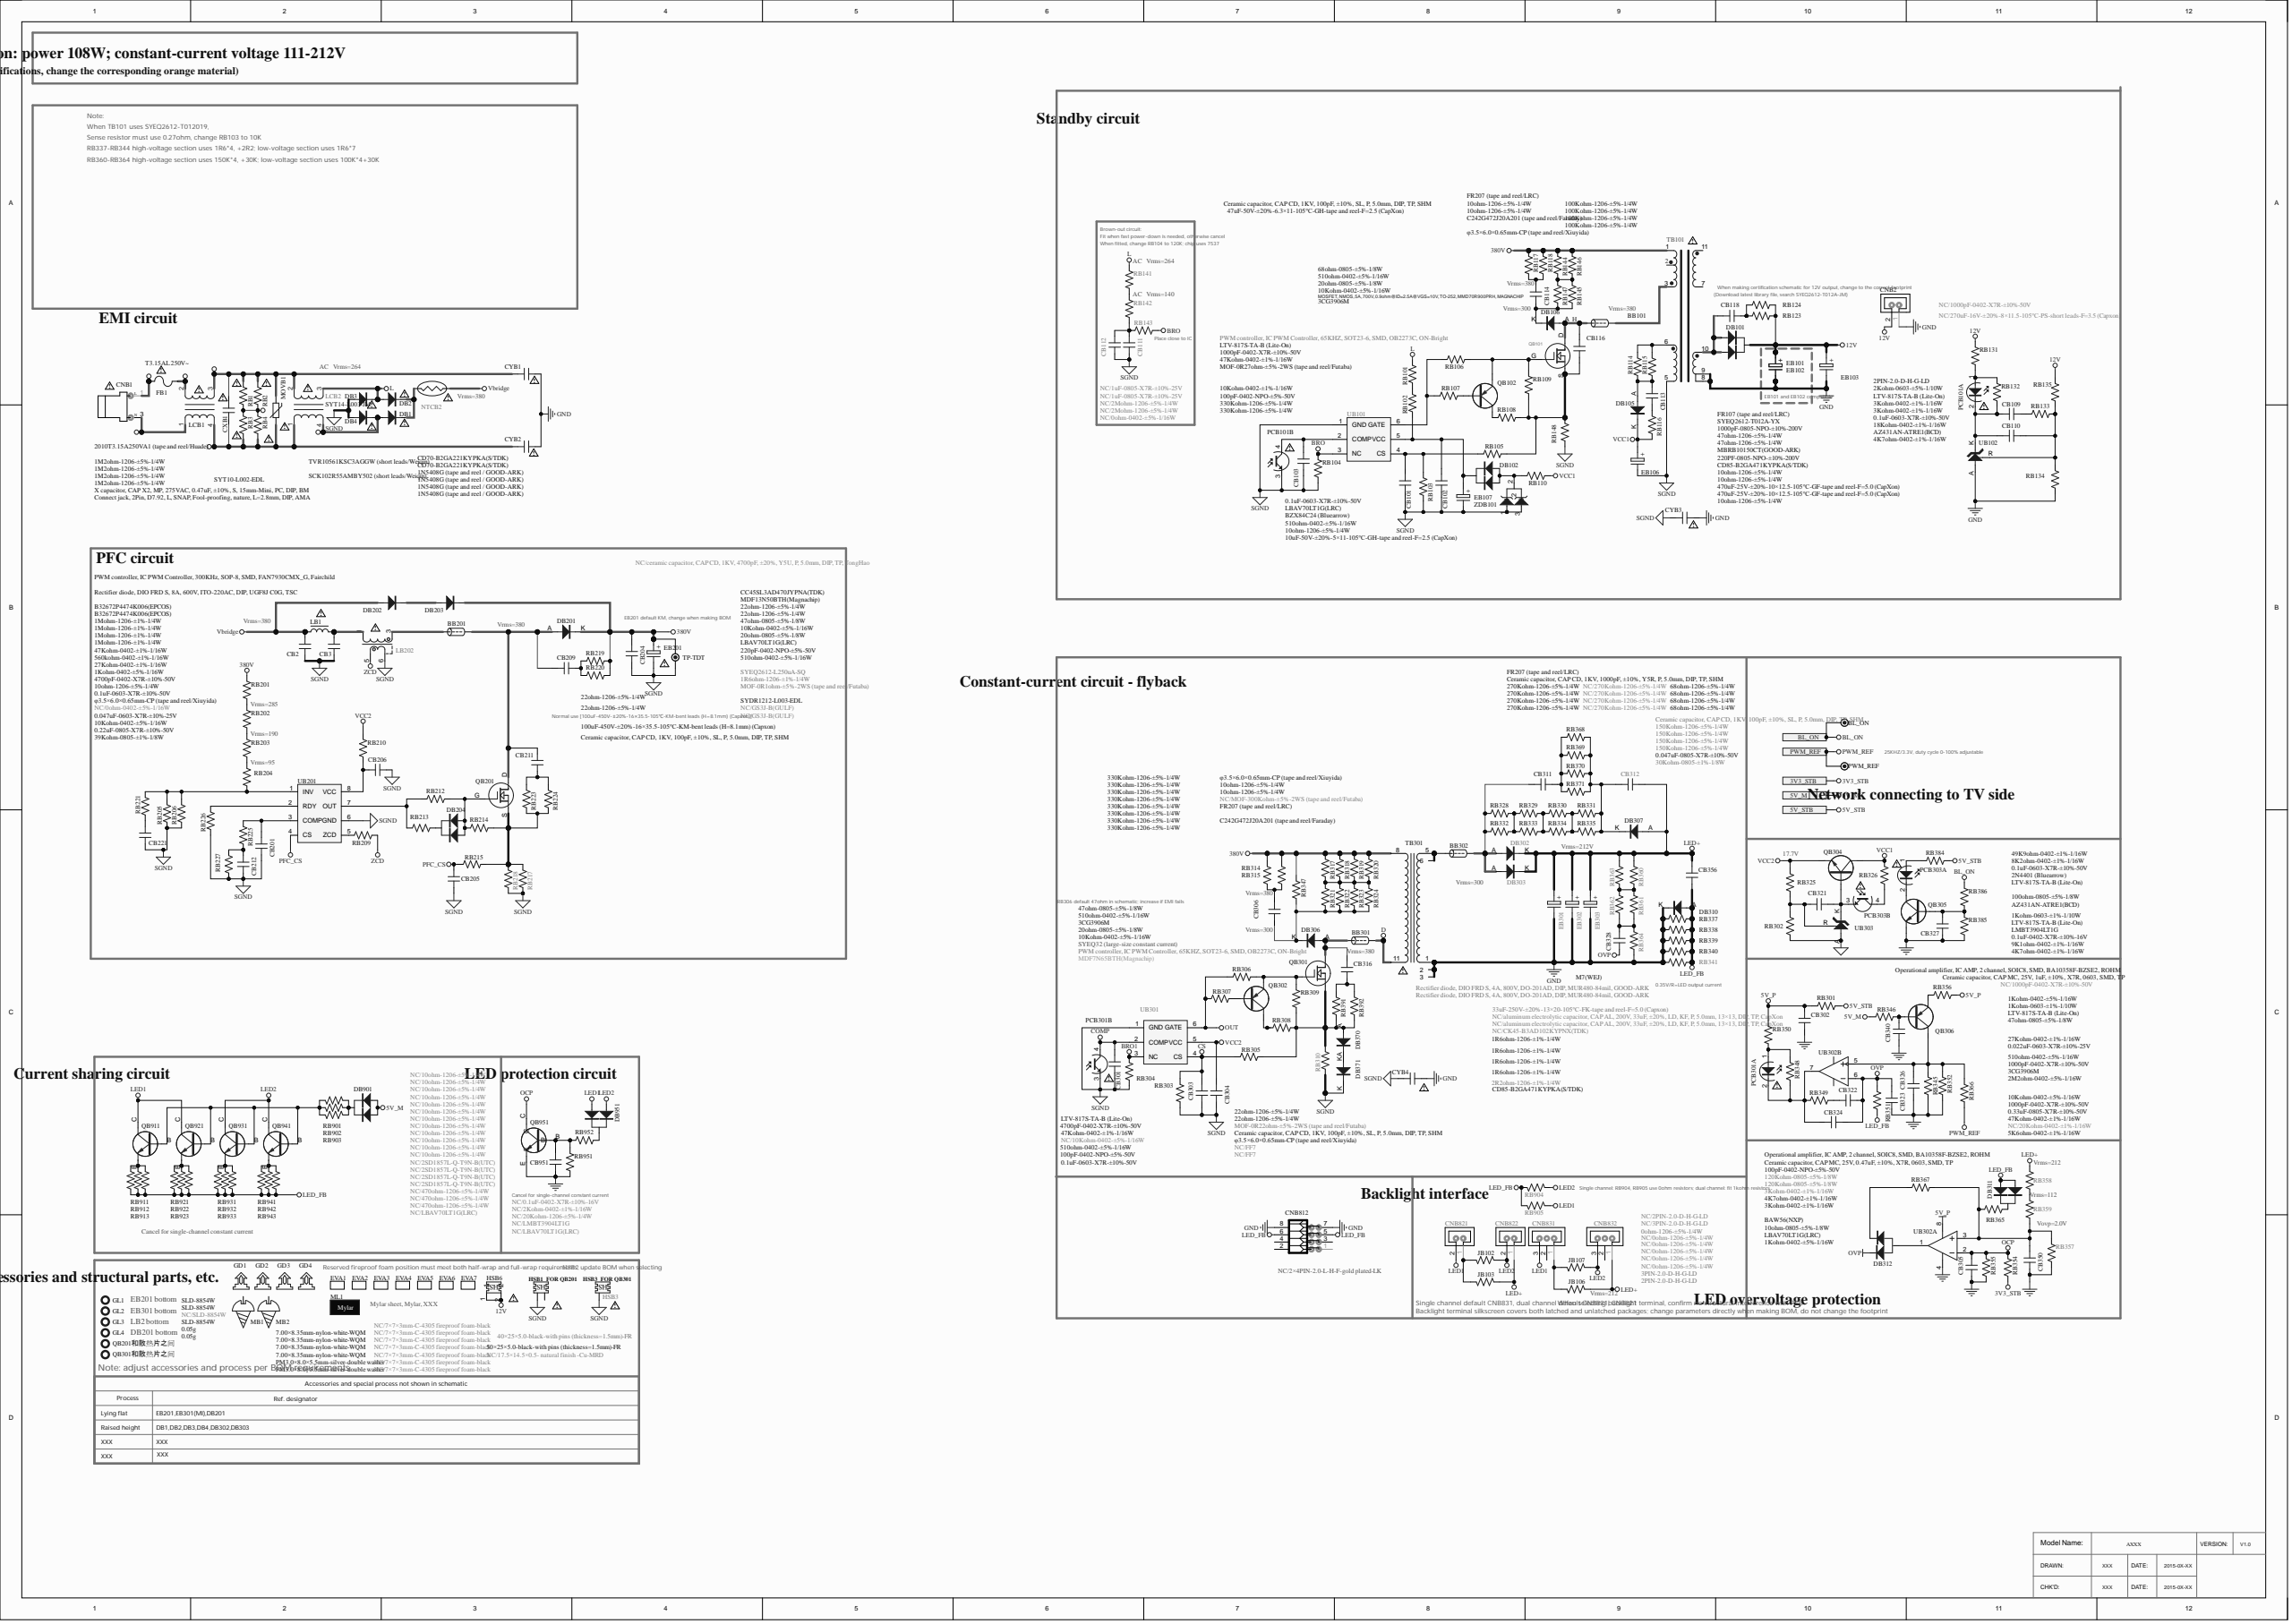Circuit board | Altium Designer | 709 parts | 378 nets | one sheet of the schematic
Parts on this sheet (reference | value | footprint):
BB101 | f3.5×6.0×0.65mm-CP (tape and reel/Xiuyida) | LB/3.5*6*15
BB201 | f3.5×6.0×0.65mm-CP (tape and reel/Xiuyida) | LB/3.5*6*12.5
BB301 | f3.5×6.0×0.65mm-CP (tape and reel/Xiuyida) | LB/3.5*6*12.5
BB302 | f3.5×6.0×0.65mm-CP (tape and reel/Xiuyida) | LB/3.5*6*12.5
CB2 | B32672P4474K006(EPCOS) | CAP18*7-V-15
CB3 | B32672P4474K006(EPCOS) | CAP18*7-V-15
CB101 | 100pF-0402-NPO-±5%-50V | C0402
CB102 | 0.1uF-0603-X7R-±10%-50V | C0603
CB103 | 1000pF-0402-X7R-±10%-50V | C0402
CB109 | 0.1uF-0603-X7R-±10%-50V | C0603
CB110 | NC/1000pF-0402-X7R-±10%-50V | C0402
CB111 | NC/1uF-0805-X7R-±10%-25V | C0805
CB112 | NC/1uF-0805-X7R-±10%-25V | C0805
CB113 | 220PF-0805-NPO-±10%-200V | C0805
CB114 | C242G472J20A201 (tape and reel/Faraday) | CAP8*2.5-V-5
CB116 | Ceramic capacitor, CAP CD, 1KV, 100pF, ±10%, SL, P, 5.0mm, DIP, TP, SHM | CAP7.5*2.5-V-5
CB118 | 1000pF-0805-NPO-±10%-200V | C0805
CB201 | 0.047uF-0603-X7R-±10%-25V | C0603
CB204 | NC/ceramic capacitor, CAP CD, 1KV, 4700pF, ±20%, Y5U, P, 5.0mm, DIP, TP, TongHao | CAP9.8*4-V-5
CB205 | 220pF-0402-NPO-±5%-50V | C0402
CB206 | 0.1uF-0603-X7R-±10%-50V | C0603
CB209 | Ceramic capacitor, CAP CD, 1KV, 100pF, ±10%, SL, P, 5.0mm, DIP, TP, SHM | CAP7.5*2.5-V-5
CB211 | CC45SL3AD470JYPNA(TDK) | CAP7.5*2.5-V-5
CB212 | 0.22uF-0805-X7R-±10%-50V | C0805
CB221 | 4700pF-0402-X7R-±10%-50V | C0402
CB301 | 4700pF-0402-X7R-±10%-50V | C0402
CB302 | Ceramic capacitor, CAP MC, 25V, 1uF, ±10%, X7R, 0603, SMD, TP | C0603
CB303 | 100pF-0402-NPO-±5%-50V | C0402
CB304 | 0.1uF-0603-X7R-±10%-50V | C0603
CB305 | 100pF-0402-NPO-±5%-50V | C0402
CB306 | C242G472J20A201 (tape and reel/Faraday) | CAP8*2.5-V-5
CB311 | Ceramic capacitor, CAP CD, 1KV, 1000pF, ±10%, Y5R, P, 5.0mm, DIP, TP, SHM | CAP7.5*2.5-V-5
CB312 | Ceramic capacitor, CAP CD, 1KV, 100pF, ±10%, SL, P, 5.0mm, DIP, TP, SHM | CAP7.5*2.5-V-5
CB316 | Ceramic capacitor, CAP CD, 1KV, 100pF, ±10%, SL, P, 5.0mm, DIP, TP, SHM | CAP7.5*2.5-V-5
CB321 | 0.1uF-0603-X7R-±10%-50V | C0603
CB322 | 0.022uF-0603-X7R-±10%-25V | C0603
CB323 | 1000pF-0402-X7R-±10%-50V | C0402
CB324 | NC/1000pF-0402-X7R-±10%-50V | C0402
CB326 | 0.33uF-0805-X7R-±10%-50V | C0805
CB327 | 0.1uF-0402-X7R-±10%-16V | C0402
CB328 | 0.047uF-0805-X7R-±10%-50V | C0805
CB340 | 1000pF-0402-X7R-±10%-50V | C0402
CB350 | Ceramic capacitor, CAP MC, 25V, 0.47uF, ±10%, X7R, 0603, SMD, TP | C0603
CB356 | NC/CK45-B3AD102KYPNX(TDK) | CAP8.5*4-V-5
CB951 | NC/0.1uF-0402-X7R-±10%-16V | C0402
CNB1 | Connect jack, 2Pin, D7.92, L, SNAP, Fool-proofing, nature, L=2.8mm, DIP, AMA | CON2-H7.92
CNB2 | 2PIN-2.0-D-H-G-LD | SIP2/2.0D-1
CNB812 | NC/2×4PIN-2.0-L-H-F-gold plated-LK | SIP2*4H/2.0DF-1
CNB821 | NC/2PIN-2.0-D-H-G-LD | SIP2/2.0D-CP
CNB822 | 2PIN-2.0-D-H-G-LD | SIP2/2.0D-CP
CNB831 | NC/3PIN-2.0-D-H-G-LD | SIP3/2.0D-CP
CNB832 | 3PIN-2.0-D-H-G-LD | SIP3/2.0D-CP
CXB1 | X capacitor, CAP X2, MP, 275VAC, 0.47uF, ±10%, S, 15mm-Mini, PC, DIP, BM | CAP18*8.5-V-15
CYB1 | CD70-B2GA221KYPKA(S/TDK) | CAP13*4.5-V-10
CYB2 | CD70-B2GA221KYPKA(S/TDK) | CAP13*4.5-V-10
CYB3 | CD85-B2GA471KYPKA(S/TDK) | CAP13*4.5-V-10
CYB4 | CD85-B2GA471KYPKA(S/TDK) | CAP13*4.5-V-10
DB1 | 1N5408G (tape and reel / GOOD-ARK) | D3-H-20
DB2 | 1N5408G (tape and reel / GOOD-ARK) | D3-H-20
DB3 | 1N5408G (tape and reel / GOOD-ARK) | D3-H-20
DB4 | 1N5408G (tape and reel / GOOD-ARK) | D3-H-20
DB101 | MBRB10150CT(GOOD-ARK) | D2PAK3
DB102 | LBAV70LT1G(LRC) | SO-23
DB105 | FR107 (tape and reel/LRC) | D1-H-12.5
DB106 | FR207 (tape and reel/LRC) | D2-H-17.5
DB201 | Rectifier diode, DIO FRD S, 8A, 600V, ITO-220AC, DIP, UGF8J C0G, TSC | TO-220-AK-H
DB202 | NC/GS3J-B(GULF) | DIODE-SMB-1
DB203 | NC/GS3J-B(GULF) | DIODE-SMB-1
DB204 | LBAV70LT1G(LRC) | SO-23
DB302 | Rectifier diode, DIO FRD S, 4A, 800V, DO-201AD, DIP, MUR480-84mil, GOOD-ARK | D3-H-20
DB303 | Rectifier diode, DIO FRD S, 4A, 800V, DO-201AD, DIP, MUR480-84mil, GOOD-ARK | D3-H-20
DB306 | FR207 (tape and reel/LRC) | D2-H-17.5
DB307 | FR207 (tape and reel/LRC) | D2-H-17.5
DB310 | M7(WEJ) | DIODE-S-2
DB311 | LBAV70LT1G(LRC) | SO-23
DB312 | BAW56(NXP) | SO-23-1
DB370 | NC/FF7 | DIODE-S-14
DB371 | NC/FF7 | DIODE-S-14
DB901 | NC/LBAV70LT1G(LRC) | SO-23
DB951 | NC/LBAV70LT1G(LRC) | SO-23
EB101 | 470uF-25V-±20%-10×12.5-105℃-GF-tape and reel-F=5.0 (CapXon) | EC(10*12.5)-V-5
EB102 | NC/270uF-16V-±20%-8×11.5-105℃-PS-short leads-F=3.5 (Capxon) | EC(8*11)-V-3.5
EB103 | 470uF-25V-±20%-10×12.5-105℃-GF-tape and reel-F=5.0 (CapXon) | EC(10*12.5)-V-5
EB106 | 47uF-50V-±20%-6.3×11-105℃-GH-tape and reel-F=2.5 (CapXon) | EC(6.3*11)-V-2.5
EB107 | 10uF-50V-±20%-5×11-105℃-GH-tape and reel-F=2.5 (CapXon) | EC(5*11)-V-2.5
EB201 | 100uF-450V-±20%-16×35.5-105℃-KM-bent leads (H=8.1mm) (Capxon) | EC(16*37)-H-7.5
EB301 | 33uF-250V-±20%-13×20-105℃-FK-tape and reel-F=5.0 (Capxon) | EC(13*20)-H-5
EB302 | NC/aluminum electrolytic capacitor, CAP AL, 200V, 33uF, ±20%, LD, KF, P, 5.0mm, 13×13, DIP, TP, CapXon | EC(13*13)-V-5
EB303 | NC/aluminum electrolytic capacitor, CAP AL, 200V, 33uF, ±20%, LD, KF, P, 5.0mm, 13×13, DIP, TP, CapXon | EC(13*13)-V-5
EVA1 | NC/7×7×3mm-C-4305 fireproof foam-black | EVA(7*7*3)
EVA2 | NC/7×7×3mm-C-4305 fireproof foam-black | EVA(7*7*3)
EVA3 | NC/7×7×3mm-C-4305 fireproof foam-black | EVA(7*7*3)
EVA4 | NC/7×7×3mm-C-4305 fireproof foam-black | EVA(7*7*3)
EVA5 | NC/7×7×3mm-C-4305 fireproof foam-black | EVA(7*7*3)
EVA6 | NC/7×7×3mm-C-4305 fireproof foam-black | EVA(7*7*3)
EVA7 | NC/7×7×3mm-C-4305 fireproof foam-black | EVA(7*7*3)
FB1 | 2010T3.15A250VA1 (tape and reel/Huade) | FUSE8.5*4-V-5
GD1 | 7.00×8.35mm-nylon-white-WQM | Fixed
GD2 | 7.00×8.35mm-nylon-white-WQM | Fixed
GD3 | 7.00×8.35mm-nylon-white-WQM | Fixed
GD4 | 7.00×8.35mm-nylon-white-WQM | Fixed
GL1 | SLD-8854W | Silica gel-20
GL2 | SLD-8854W | Silica gel-10
GL3 | NC/SLD-8854W | Silica gel-10
GL4 | SLD-8854W | Silica gel-10
HSB2 | 40×25×5.0-black-with pins (thickness=1.5mm)-FR | HS018
HSB3 | 50×25×5.0-black-with pins (thickness=1.5mm)-FR | HS033
HSB6 | NC/17.5×14.5×0.5- natural finish -Cu-MRD | HS038
JB102 | NC/0ohm-1206-±5%-1/4W | R1206
JB103 | NC/0ohm-1206-±5%-1/4W | R1206
JB106 | NC/0ohm-1206-±5%-1/4W | R1206
JB107 | NC/0ohm-1206-±5%-1/4W | R1206
LB1 | SYDR1212-L003-EDL | L/LC2/15*14.5-V7.5
LB202 | SYEQ2612-L250uA-SQ | T/EQ2512*11
LCB1 | SYT10-L002-EDL | L/LC4/13.5*10-V-7*6
LCB2 | SYT14-L003-JM | L/LC4/T14-H-8*6
MB1 | PM3.0×8.0×5.5mm-silver-double washer | SCREW
MB2 | PM3.0×8.0×5.5mm-silver-double washer | SCREW
ML1 | Mylar sheet, Mylar, XXX | Mylar
MOVB1 | TVR10561KSC3AGGW (short leads/Weiqin) | VR(13*5)-V-7.5
NTCB2 | SCK102R55AMBY502 (short leads/Weiqin) | NTC(10*5)-V5
QB101 | MOSFET, NMOS, 5A, 700V, 0.9ohm@ID=2.5A@VGS=10V, TO-252, MMD70R900PRH, MAGNACHIP | TO-252-GDS
QB102 | 3CG3906M | SOT-23
QB201 | MDF13N50BTH(Magnachip) | TO-220-GDS-H
QB201和散热片之间 | 0.05g | PCB_TIME
QB301 | MDF7N65BTH(Magnachip) | TO-220-GDS-H
QB301和散热片之间 | 0.05g | PCB_TIME
QB302 | 3CG3906M | SOT-23
QB304 | 2N4401 (Bluearrow) | TO-92-EBC
QB305 | LMBT3904LT1G | SOT-23
QB306 | 3CG3906M | SOT-23
QB911 | NC/2SD1857L-Q-T9N-B(UTC) | TO-92-ECB
QB921 | NC/2SD1857L-Q-T9N-B(UTC) | TO-92-ECB
QB931 | NC/2SD1857L-Q-T9N-B(UTC) | TO-92-ECB
QB941 | NC/2SD1857L-Q-T9N-B(UTC) | TO-92-ECB
QB951 | NC/LMBT3904LT1G | SOT-23
RB1 | 1M2ohm-1206-±5%-1/4W | R1206
RB2 | 1M2ohm-1206-±5%-1/4W | R1206
RB3 | 1M2ohm-1206-±5%-1/4W | R1206
RB4 | 1M2ohm-1206-±5%-1/4W | R1206
RB101 | 330Kohm-1206-±5%-1/4W | R1206
RB102 | 330Kohm-1206-±5%-1/4W | R1206
RB103 | 10Kohm-0402-±1%-1/16W | R0402
RB104 | 47Kohm-0402-±1%-1/16W | R0402
RB105 | 510ohm-0402-±5%-1/16W | R0402
RB106 | 68ohm-0805-±5%-1/8W | R0805
RB107 | 510ohm-0402-±5%-1/16W | R0402
RB108 | 20ohm-0805-±5%-1/8W | R0805
RB109 | 10Kohm-0402-±5%-1/16W | R0402
RB110 | 10ohm-1206-±5%-1/4W | R1206
RB114 | 10ohm-1206-±5%-1/4W | R1206
RB115 | 10ohm-1206-±5%-1/4W | R1206
RB116 | 10ohm-1206-±5%-1/4W | R1206
RB117 | 10ohm-1206-±5%-1/4W | R1206
RB118 | 10ohm-1206-±5%-1/4W | R1206
RB123 | 47ohm-1206-±5%-1/4W | R1206
RB124 | 47ohm-1206-±5%-1/4W | R1206
RB131 | 2Kohm-0603-±5%-1/10W | R0603
RB132 | 3Kohm-0402-±1%-1/16W | R0402
RB133 | 3Kohm-0402-±1%-1/16W | R0402
RB134 | 4K7ohm-0402-±1%-1/16W | R0402
RB135 | 18Kohm-0402-±1%-1/16W | R0402
RB141 | NC/2Mohm-1206-±5%-1/4W | R1206
RB142 | NC/2Mohm-1206-±5%-1/4W | R1206
RB143 | NC/0ohm-0402-±5%-1/16W | R0402
RB144 | 100Kohm-1206-±5%-1/4W | R1206
RB145 | 100Kohm-1206-±5%-1/4W | R1206
RB146 | 100Kohm-1206-±5%-1/4W | R1206
RB147 | 100Kohm-1206-±5%-1/4W | R1206
RB148 | MOF-0R27ohm-±5%-2WS (tape and reel/Futaba) | R2-H-17.5
RB201 | 1Mohm-1206-±1%-1/4W | R1206
RB202 | 1Mohm-1206-±1%-1/4W | R1206
RB203 | 1Mohm-1206-±1%-1/4W | R1206
RB204 | 1Mohm-1206-±1%-1/4W | R1206
RB205 | 560kohm-0402-±1%-1/16W | R0402
RB206 | 27Kohm-0402-±1%-1/16W | R0402
RB209 | 39Kohm-0805-±1%-1/8W | R0805
RB210 | 10ohm-1206-±5%-1/4W | R1206
RB212 | 47ohm-0805-±5%-1/8W | R0805
RB213 | 20ohm-0805-±5%-1/8W | R0805
RB214 | 10Kohm-0402-±5%-1/16W | R0402
RB215 | 510ohm-0402-±5%-1/16W | R0402
RB217 | MOF-0R1ohm-±5%-2WS (tape and reel/Futaba) | R2-H-17.5
RB218 | 1R6ohm-1206-±1%-1/4W | R1206
RB219 | 22ohm-1206-±5%-1/4W | R1206
RB220 | 22ohm-1206-±5%-1/4W | R1206
RB221 | 1Kohm-0402-±5%-1/16W | R0402
RB223 | 22ohm-1206-±5%-1/4W | R1206
RB224 | 22ohm-1206-±5%-1/4W | R1206
RB225 | 10Kohm-0402-±5%-1/16W | R0402
RB226 | 47Kohm-0402-±1%-1/16W | R0402
RB227 | NC/0ohm-0402-±5%-1/16W | R0402
RB301 | 47ohm-0805-±5%-1/8W | R0805
RB302 | 8K2ohm-0402-±1%-1/16W | R0402
RB303 | NC/10Kohm-0402-±5%-1/16W | R0402
RB304 | 47Kohm-0402-±1%-1/16W | R0402
RB305 | 510ohm-0402-±5%-1/16W | R0402
RB306 | 47ohm-0805-±5%-1/8W | R0805
RB307 | 510ohm-0402-±5%-1/16W | R0402
RB308 | 20ohm-0805-±5%-1/8W | R0805
RB309 | 10Kohm-0402-±5%-1/16W | R0402
RB310 | MOF-0R22ohm-±5%-2WS (tape and reel/Futaba) | R2-H-17.5
RB314 | 10ohm-1206-±5%-1/4W | R1206
RB315 | 10ohm-1206-±5%-1/4W | R1206
RB317 | 330Kohm-1206-±5%-1/4W | R1206
RB318 | 330Kohm-1206-±5%-1/4W | R1206
RB319 | 330Kohm-1206-±5%-1/4W | R1206
RB320 | 330Kohm-1206-±5%-1/4W | R1206
RB321 | 330Kohm-1206-±5%-1/4W | R1206
RB322 | 330Kohm-1206-±5%-1/4W | R1206
RB323 | 330Kohm-1206-±5%-1/4W | R1206
RB324 | 330Kohm-1206-±5%-1/4W | R1206
RB325 | 49K9ohm-0402-±1%-1/16W | R0402
RB326 | 100ohm-0805-±5%-1/8W | R0805
RB328 | 270Kohm-1206-±5%-1/4W | R1206
RB329 | 270Kohm-1206-±5%-1/4W | R1206
RB330 | 270Kohm-1206-±5%-1/4W | R1206
RB331 | 270Kohm-1206-±5%-1/4W | R1206
RB332 | NC/270Kohm-1206-±5%-1/4W | R1206
RB333 | NC/270Kohm-1206-±5%-1/4W | R1206
RB334 | NC/270Kohm-1206-±5%-1/4W | R1206
RB335 | NC/270Kohm-1206-±5%-1/4W | R1206
RB337 | 1R6ohm-1206-±1%-1/4W | R1206
RB338 | 1R6ohm-1206-±1%-1/4W | R1206
RB339 | 1R6ohm-1206-±1%-1/4W | R1206
RB340 | 1R6ohm-1206-±1%-1/4W | R1206
RB341 | 2R2ohm-1206-±1%-1/4W | R1206
RB345 | 5K6ohm-0402-±1%-1/16W | R0402
RB346 | 510ohm-0402-±5%-1/16W | R0402
RB347 | NC/MOF-300Kohm-±5%-2WS (tape and reel/Futaba) | R2-H-17.5
RB348 | 1Kohm-0402-±5%-1/16W | R0402
RB349 | 27Kohm-0402-±1%-1/16W | R0402
RB350 | 1Kohm-0603-±1%-1/10W | R0603
RB351 | 10Kohm-0402-±5%-1/16W | R0402
RB352 | NC/20Kohm-0402-±1%-1/16W | R0402
RB354 | 3Kohm-0402-±1%-1/16W | R0402
RB355 | 4K7ohm-0402-±1%-1/16W | R0402
RB356 | 2M2ohm-0402-±5%-1/16W | R0402
RB357 | 3Kohm-0402-±1%-1/16W | R0402
RB358 | 120Kohm-0805-±5%-1/8W | R0805
RB359 | 120Kohm-0805-±5%-1/8W | R0805
RB360 | 150Kohm-1206-±5%-1/4W | R1206
RB361 | 150Kohm-1206-±5%-1/4W | R1206
RB362 | 150Kohm-1206-±5%-1/4W | R1206
RB363 | 150Kohm-1206-±5%-1/4W | R1206
RB364 | 30Kohm-0805-±1%-1/8W | R0805
RB365 | 10ohm-0805-±5%-1/8W | R0805
RB366 | 47Kohm-0402-±1%-1/16W | R0402
RB367 | 1Kohm-0402-±5%-1/16W | R0402
RB368 | 68ohm-1206-±5%-1/4W | R1206
RB369 | 68ohm-1206-±5%-1/4W | R1206
RB370 | 68ohm-1206-±5%-1/4W | R1206
RB371 | 68ohm-1206-±5%-1/4W | R1206
RB384 | 1Kohm-0603-±1%-1/10W | R0603
RB385 | 4K7ohm-0402-±1%-1/16W | R0402
RB386 | 9K1ohm-0402-±1%-1/16W | R0402
RB391 | 22ohm-1206-±5%-1/4W | R1206
RB392 | 22ohm-1206-±5%-1/4W | R1206
RB901 | NC/470ohm-1206-±5%-1/4W | R1206
RB902 | NC/470ohm-1206-±5%-1/4W | R1206
RB903 | NC/470ohm-1206-±5%-1/4W | R1206
RB904 | 0ohm-1206-±5%-1/4W | R1206
RB905 | NC/0ohm-1206-±5%-1/4W | R1206
RB911 | NC/10ohm-1206-±5%-1/4W | R1206
RB912 | NC/10ohm-1206-±5%-1/4W | R1206
RB913 | NC/10ohm-1206-±5%-1/4W | R1206
RB921 | NC/10ohm-1206-±5%-1/4W | R1206
RB922 | NC/10ohm-1206-±5%-1/4W | R1206
RB923 | NC/10ohm-1206-±5%-1/4W | R1206
RB931 | NC/10ohm-1206-±5%-1/4W | R1206
RB932 | NC/10ohm-1206-±5%-1/4W | R1206
RB933 | NC/10ohm-1206-±5%-1/4W | R1206
RB941 | NC/10ohm-1206-±5%-1/4W | R1206
RB942 | NC/10ohm-1206-±5%-1/4W | R1206
RB943 | NC/10ohm-1206-±5%-1/4W | R1206
RB951 | NC/2Kohm-0402-±1%-1/16W | R0402
RB952 | NC/20Kohm-1206-±5%-1/4W | R1206
TB101 | SYEQ2612-T012A-YX | T/EQ2512*11
TB301 | SYEQ32 (large-size constant current) | T/EQ3214*11
TP-TDT | TP-TDT
UB101 | PWM controller, IC PWM Controller, 65KHZ, SOT23-6, SMD, OB2273C, ON-Bright | SOT-26
UB102 | AZ431AN-ATRE1(BCD) | SOT-23-RAK
UB201 | PWM controller, IC PWM Controller, 300KHz, SOP-8, SMD, FAN7930CMX_G, Fairchild | SO-8A
UB301 | PWM controller, IC PWM Controller, 65KHZ, SOT23-6, SMD, OB2273C, ON-Bright | SOT-26
UB303 | AZ431AN-ATRE1(BCD) | SOT-23-RAK
ZDB101 | BZX84C24 (Bluearrow) | SO-23
Nets of these parts (net: part-pin ...):
ZCD: LB202-5 RB209-2
VCC2: CB304-1 QB304-E RB210-2 RB325-2 UB301-5
VCC1: DB105-K EB106-1 QB304-C RB110-2 RB116-1 RB326-1
Vbridge: CB2-1 DB202-A LB1-1 NTCB2-1
SGND: CB2-2 CB3-2 CB101-2 CB102-2 CB103-2 CB111-1 CB112-1 CB201-1 CB204-1 CB205-1 CB206-1 CB212-2 CB221-1 CB301-1 CB303-2 CB304-2 CYB3-1 CYB4-1 DB3-A DB4-A DB371-K EB106-2 EB107-2 EB201-2 HSB2-3 HSB3-1 LB202-6 RB103-1 RB104-1 RB148-1 RB205-1 RB206-2 RB217-1 RB218-1 RB226-1 RB227-1 RB302-2 RB303-2 RB304-2 RB310-1 TB101-5 TP-TDT-2 UB101-1 UB201-6 UB301-1 UB303-A ZDB101-1 ZDB101-3
PWM_REF: RB366-2
PFC_CS: CB205-2 RB215-1 UB201-4
OVP: CB322-2 CB323-2 CB324-2 CB328-1 DB312-2 RB351-2
OUT: RB306-1 RB307-1 UB301-6
OCP: CB305-1 QB951-C RB354-1 RB355-1
NetRB360_1: RB360-1 RB361-2 RB362-2 RB363-1
NetRB358_2: RB358-2 RB359-1
NetRB330_2: RB330-2 RB331-1 RB334-2 RB335-1
NetRB329_2: RB329-2 RB330-1 RB333-2 RB334-1
NetRB328_2: RB328-2 RB329-1 RB332-2 RB333-1
NetRB317_1: RB317-1 RB318-1 RB319-1 RB320-1 RB321-2 RB322-2 RB323-2 RB324-2
NetRB226_2: RB226-2 UB201-2
NetRB212_1: RB212-1 RB213-1 UB201-7
NetRB209_1: RB209-1 UB201-5
NetRB204_2: RB204-2 RB205-2 RB206-1 RB221-2 UB201-1
NetRB203_2: RB203-2 RB204-1
NetRB202_2: RB202-2 RB203-1
NetRB201_2: RB201-2 RB202-1
NetRB144_2: RB144-2 RB145-1 RB146-2 RB147-1
NetRB141_1: RB141-1 RB142-2
NetRB114_2: RB114-2 RB115-2 TB101-6
NetRB106_1: RB106-1 RB107-1 UB101-6
NetRB101_2: RB101-2 RB102-1
NetQB941_E: QB941-E RB941-2 RB942-2 RB943-2
NetQB931_E: QB931-E RB931-2 RB932-2 RB933-2
NetQB921_E: QB921-E RB921-2 RB922-2 RB923-2
NetQB911_E: QB911-E RB911-2 RB912-2 RB913-2
NetQB911_B: QB911-B QB921-B QB931-B QB941-B RB901-1 RB902-1 RB903-1
NetQB306_E: QB306-E RB356-1
NetQB302_C: QB302-C RB308-1
NetQB302_B: QB302-B RB307-2
NetQB301_G: QB301-G QB302-E RB306-2 RB309-2
NetQB201_S: QB201-S RB214-1 RB215-2 RB217-2 RB218-2 RB223-2 RB224-2
NetQB102_C: QB102-C RB108-1
NetQB102_B: QB102-B RB107-2
NetQB101_G: QB101-G QB102-E RB106-2 RB109-1
NetPCB303_4: RB326-2
NetPCB303_2: QB305-C
NetPCB303_1: RB384-2
NetPCB301_1: RB348-1 RB350-1
NetPCB101_1: RB131-2 RB132-1
NetDB951_2: DB951-2 RB952-2
NetDB901_2: DB901-2 RB901-2 RB902-2 RB903-2
NetDB370_K: DB370-K DB371-A
NetDB370_A: DB370-A QB301-S RB305-2 RB308-2 RB309-1 RB310-2 RB391-2 RB392-2
NetDB312_3: DB312-3
NetDB312_1: DB312-1 RB367-1
NetDB311_2: DB311-2 RB365-1
NetDB204_2: DB204-2 RB213-2
NetDB204_1: DB204-1 DB204-3 QB201-G RB212-2 RB214-2
NetDB202_K: DB202-K DB203-A
NetDB102_1: DB102-1 DB102-3 RB110-1 ZDB101-2
NetDB1_K: DB1-K DB2-K NTCB2-2
NetCNB831_1: CNB831-1 JB106-2 JB107-2
NetCNB821_1: CNB821-1 JB102-1 JB103-2
NetCB951_1: CB951-1 QB951-B RB951-2 RB952-1
NetCB350_2: CB350-2 RB357-2 RB359-2 RB365-2 RB367-2
NetCB340_1: CB340-1 QB306-B RB346-2
NetCB328_2: CB328-2 RB361-1 RB362-1 RB364-2
NetCB327_1: CB327-1 QB305-B RB385-2 RB386-1
NetCB326_1: CB326-1 QB306-C RB345-1 RB352-1 RB366-1
NetCB324_1: CB324-1 RB348-2 RB349-1
NetCB322_1: CB322-1 RB349-2
NetCB321_2: CB321-2 RB302-1 RB325-1 UB303-R
NetCB321_1: CB321-1 QB304-B UB303-K
NetCB316_1: CB316-1 RB391-1 RB392-1
NetCB312_1: CB312-1 DB307-K RB331-2 RB335-2 RB368-2 RB369-2 RB370-2 RB371-2
NetCB311_2: CB311-2 RB368-1 RB369-1 RB370-1 RB371-1
NetCB306_2: CB306-2 DB306-K RB321-1 RB322-1 RB323-1 RB324-1 RB347-1
NetCB306_1: CB306-1 RB314-1 RB315-1
NetCB221_2: CB221-2 RB221-1
NetCB212_1: CB212-1 RB225-2 RB227-2
NetCB211_2: CB211-2 RB223-1 RB224-1
NetCB209_1: CB209-1 RB219-1 RB220-1
NetCB206_2: CB206-2 RB210-1 UB201-8
NetCB201_2: CB201-2 RB225-1 UB201-3
NetCB118_2: CB118-2 RB123-1 RB124-1
NetCB118_1: CB118-1 DB101-1 DB101-3 TB101-10
NetCB116_1: CB116-1 QB101-S RB105-2 RB108-2 RB109-2 RB148-2
NetCB114_2: CB114-2 DB106-K RB145-2 RB147-2
NetCB114_1: CB114-1 RB117-2 RB118-2
NetCB113_2: CB113-2 RB116-2
NetCB113_1: CB113-1 DB105-A RB114-1 RB115-1
NetCB111_2: CB111-2 CB112-2 RB142-1 RB143-1
NetCB110_2: CB110-2 RB133-2 RB134-1 RB135-2 UB102-R
NetCB109_2: CB109-2 RB133-1
NetCB109_1: CB109-1 CB110-1 RB132-2 UB102-K
NetCB103_1: CB103-1 UB101-2
NetCB102_1: CB102-1 DB102-2 EB107-1 RB102-2 UB101-5
NetCB101_1: CB101-1 RB103-2 RB105-1 UB101-4
NetCB3_1: CB3-1 LB1-2 LB202-1
NetBB302_2: BB302-2 CB311-1 DB302-A DB303-A RB328-1 RB332-1
NetBB302_1: BB302-1 TB301-5 TB301-6
NetBB301_1: BB301-1 CB316-2 DB306-A QB301-D
NetBB201_2: BB201-2 CB209-2 CB211-1 DB201-A QB201-D
NetBB201_1: BB201-1 LB202-3
NetBB101_2: BB101-2 TB101-3
N-3: DB2-A DB3-K LCB2-4
N-2: CXB1-2 CYB2-2 LCB1-4 LCB2-1 MOVB1-1 RB3-2 RB4-2
N-1: CNB1-3 LCB1-1
LED_FB: CB356-1 CNB812-5 CNB812-6 DB310-A DB311-1 DB311-3 RB337-2 RB338-2 RB339-2 RB340-2 RB341-2 RB351-1 RB904-2 RB905-2 RB911-1 RB912-1 RB913-1 RB921-1 RB922-1 RB923-1 RB931-1 RB932-1 RB933-1 RB941-1 RB942-1 RB943-1
LED+: CB312-2 CB356-2 CNB822-1 CNB832-1 DB302-K DB303-K DB307-A EB301-1 EB302-1 EB303-1 JB103-1 JB106-1 RB358-1 RB360-2 RB363-2
LED2: CNB822-2 CNB832-3 DB951-1 JB102-2 JB107-1 QB931-C QB941-C RB904-1
LED1: CNB821-2 CNB831-3 DB951-3 QB911-C QB921-C RB905-1
L-N: RB1-2 RB2-2 RB3-1 RB4-1
L-3: CXB1-1 CYB1-2 LCB1-3 LCB2-2 MOVB1-2 RB1-1 RB2-1
L-2: FB1-2 LCB1-2
L-1: CNB1-1 FB1-1
L: DB1-A DB4-K LCB2-3 RB101-1 RB141-2
H: BB101-1 CB116-2 DB106-A QB101-D
GND: CB302-1 CB305-2 CB323-1 CB326-2 CB327-2 CB340-2 CB350-1 CB951-2 CNB2-1 CNB812-7 CNB812-8 CYB1-1 CYB2-1 CYB3-2 CYB4-2 DB310-K EB101-2 EB102-2 EB103-2 EB301-2 EB302-2 EB303-2 QB305-E QB951-E RB134-2 RB337-1 RB338-1 RB339-1 RB340-1 RB341-1 RB345-2 RB352-2 RB355-2 RB357-1 RB364-1 RB385-1 RB951-1 TB101-8 TB101-9 TB301-1 TB301-2 TB301-3 UB102-A
D: BB301-2 TB301-11
CS: CB303-1 RB303-1 RB305-1 UB301-4
COMP: CB301-2 UB301-2
BRO1: RB304-1 UB301-3
BRO: RB104-2 RB143-2 UB101-3
BL_ON: RB386-2
380V: CB204-2 DB201-K DB203-K EB201-1 RB117-1 RB118-1 RB144-1 RB146-1 RB201-1 RB219-2 RB220-2 RB314-2 RB315-2 RB317-2 RB318-2 RB319-2 RB320-2 RB347-2 TB101-1 TB301-8 TP-TDT-1
12V: CNB2-2 DB101-2 EB101-1 EB102-1 EB103-1 HSB6-1 HSB6-2 RB123-2 RB124-2 RB131-1 RB135-1
5V_STB: RB301-2 RB384-1
5V_P: CB302-2 RB301-1 RB350-2 RB356-2
5V_M: DB901-1 DB901-3 RB346-1
3V3_STB: RB354-2